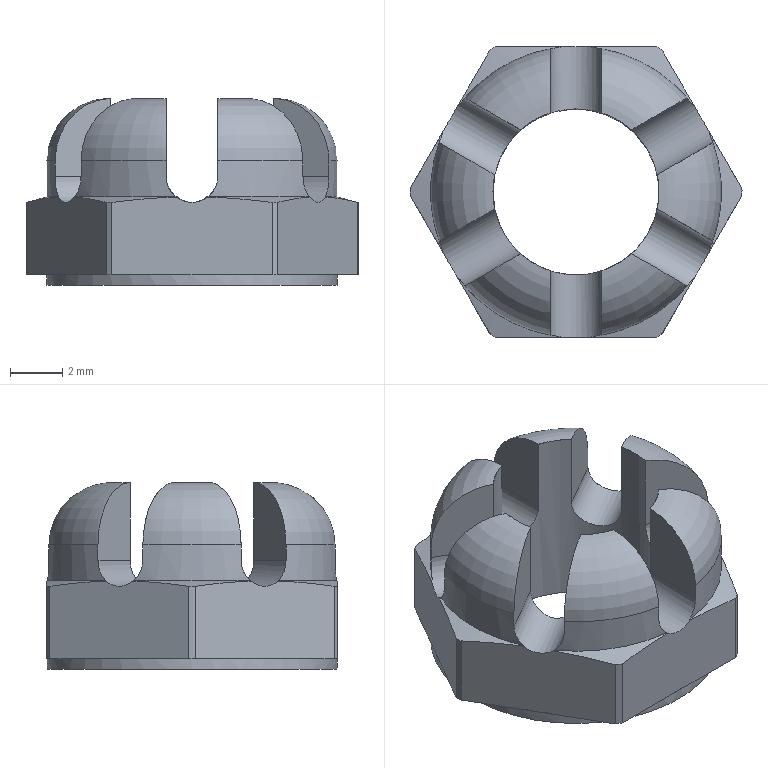Part | NX | features solid 2 | 1 solid | 63 faces | box 12.7 x 11.125 x 7.144 mm | volume 365.256 mm3 | plane 31 | cylinder 20 | torus 6 | cone 6 | commonest cylinder face diameters 11.125 x7 1.984 x6 12.7 x6 6.35 x1